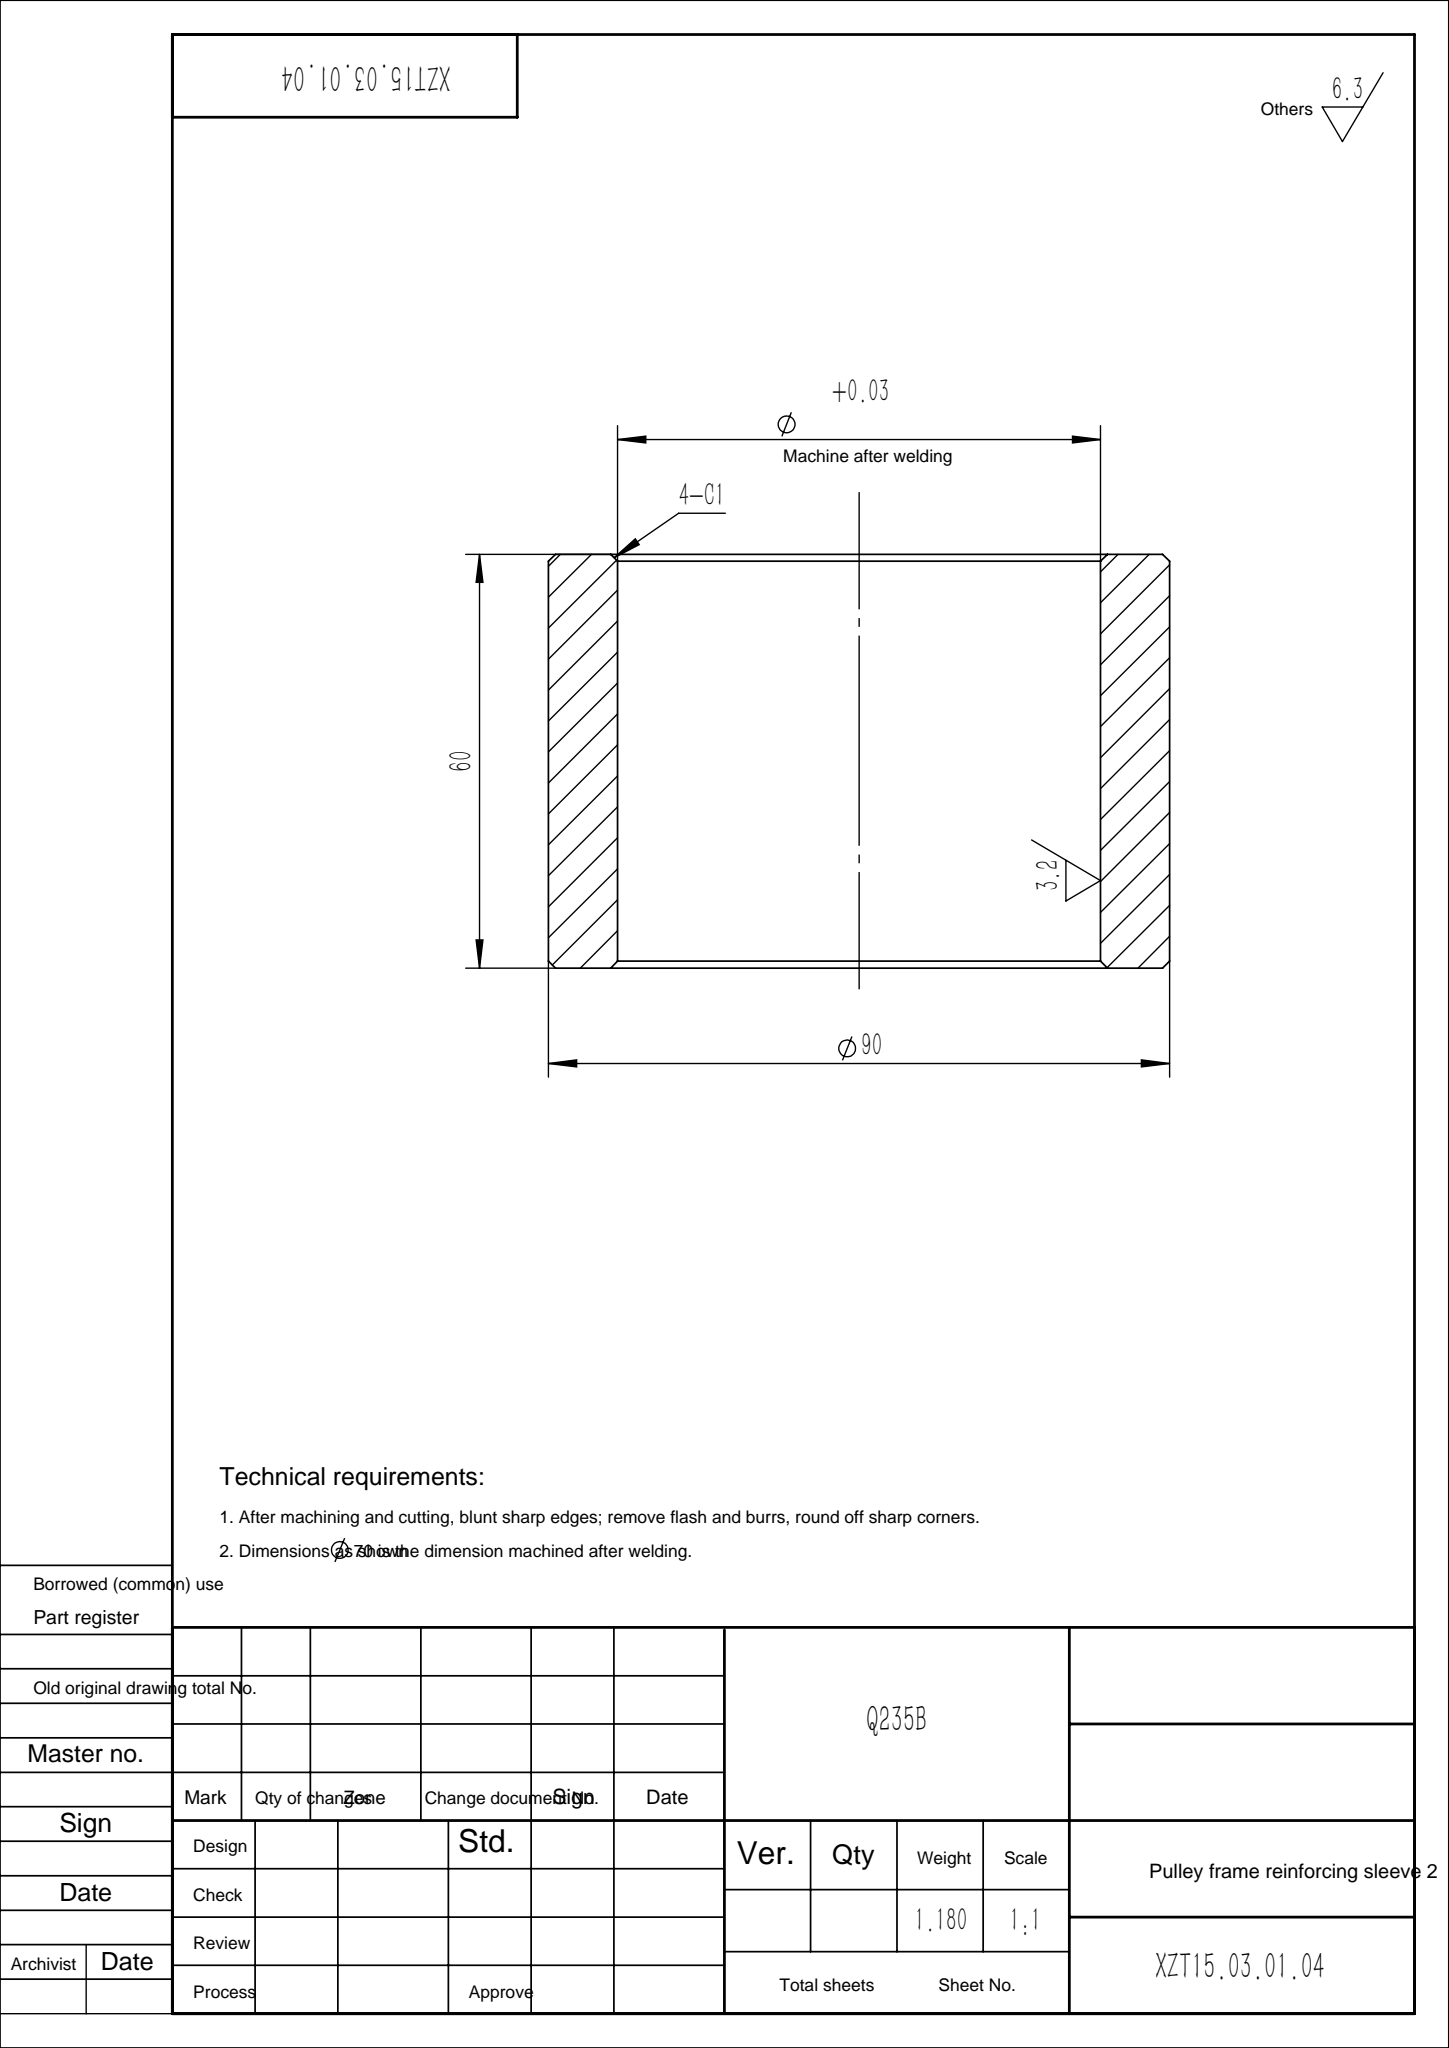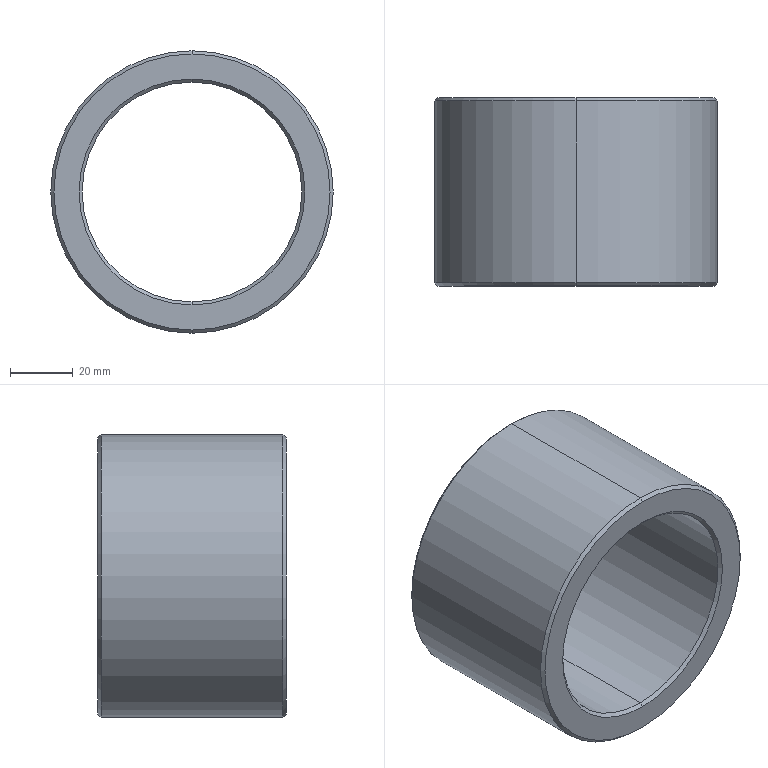Part | SolidWorks | features Chamfer 1, Extrusion 1 | 1 solid | 14 faces | box 90 x 60 x 90 mm | volume 150294 mm3 | cone 8 | cylinder 4 | plane 2 | commonest cylinder face diameters 70 x2 90 x2
STEP:
#1=CARTESIAN_POINT('',(0.,60.,44.));
#2=VERTEX_POINT('',#1);
#3=CARTESIAN_POINT('',(0.,60.,-44.));
#4=VERTEX_POINT('',#3);
#5=CARTESIAN_POINT('',(0.,60.,0.));
#6=DIRECTION('',(0.,1.,0.));
#7=DIRECTION('',(0.,0.,1.));
#8=AXIS2_PLACEMENT_3D('',#5,#6,#7);
#9=CIRCLE('',#8,44.);
#10=EDGE_CURVE('',#2,#4,#9,.T.);
#11=ORIENTED_EDGE('',*,*,#10,.F.);
#12=CARTESIAN_POINT('',(0.,59.,45.));
#13=VERTEX_POINT('',#12);
#14=CARTESIAN_POINT('',(0.,60.,44.));
#15=DIRECTION('',(0.,-0.7071,0.7071));
#16=VECTOR('',#15,1000.);
#17=LINE('',#14,#16);
#18=EDGE_CURVE('',#2,#13,#17,.T.);
#19=ORIENTED_EDGE('',*,*,#18,.T.);
#20=CARTESIAN_POINT('',(0.,59.,-45.));
#21=VERTEX_POINT('',#20);
#22=CARTESIAN_POINT('',(0.,59.,0.));
#23=DIRECTION('',(0.,-1.,0.));
#24=DIRECTION('',(0.,0.,1.));
#25=AXIS2_PLACEMENT_3D('',#22,#23,#24);
#26=CIRCLE('',#25,45.);
#27=EDGE_CURVE('',#21,#13,#26,.T.);
#28=ORIENTED_EDGE('',*,*,#27,.F.);
#29=CARTESIAN_POINT('',(0.,60.,-44.));
#30=DIRECTION('',(0.,-0.7071,-0.7071));
#31=VECTOR('',#30,1000.);
#32=LINE('',#29,#31);
#33=EDGE_CURVE('',#4,#21,#32,.T.);
#34=ORIENTED_EDGE('',*,*,#33,.F.);
#35=EDGE_LOOP('',(#11,#19,#28,#34));
#36=FACE_OUTER_BOUND('',#35,.T.);
#37=CARTESIAN_POINT('',(0.,60.,0.));
#38=DIRECTION('',(0.,-1.,0.));
#39=DIRECTION('',(0.,0.,-1.));
#40=AXIS2_PLACEMENT_3D('',#37,#38,#39);
#41=CONICAL_SURFACE('',#40,44.,0.7854);
#42=ADVANCED_FACE('',(#36),#41,.T.);
#43=CARTESIAN_POINT('',(0.,0.,-44.));
#44=VERTEX_POINT('',#43);
#45=CARTESIAN_POINT('',(0.,0.,44.));
#46=VERTEX_POINT('',#45);
#47=CARTESIAN_POINT('',(0.,0.,0.));
#48=DIRECTION('',(0.,-1.,0.));
#49=DIRECTION('',(0.,0.,1.));
#50=AXIS2_PLACEMENT_3D('',#47,#48,#49);
#51=CIRCLE('',#50,44.);
#52=EDGE_CURVE('',#44,#46,#51,.T.);
#53=ORIENTED_EDGE('',*,*,#52,.F.);
#54=CARTESIAN_POINT('',(0.,1.,-45.));
#55=VERTEX_POINT('',#54);
#56=CARTESIAN_POINT('',(0.,1.,-45.));
#57=DIRECTION('',(0.,0.7071,-0.7071));
#58=VECTOR('',#57,1000.);
#59=LINE('',#56,#58);
#60=EDGE_CURVE('',#44,#55,#59,.T.);
#61=ORIENTED_EDGE('',*,*,#60,.T.);
#62=CARTESIAN_POINT('',(0.,1.,45.));
#63=VERTEX_POINT('',#62);
#64=CARTESIAN_POINT('',(0.,1.,0.));
#65=DIRECTION('',(0.,1.,0.));
#66=DIRECTION('',(0.,0.,1.));
#67=AXIS2_PLACEMENT_3D('',#64,#65,#66);
#68=CIRCLE('',#67,45.);
#69=EDGE_CURVE('',#63,#55,#68,.T.);
#70=ORIENTED_EDGE('',*,*,#69,.F.);
#71=CARTESIAN_POINT('',(0.,1.,45.));
#72=DIRECTION('',(0.,0.7071,0.7071));
#73=VECTOR('',#72,1000.);
#74=LINE('',#71,#73);
#75=EDGE_CURVE('',#46,#63,#74,.T.);
#76=ORIENTED_EDGE('',*,*,#75,.F.);
#77=EDGE_LOOP('',(#53,#61,#70,#76));
#78=FACE_OUTER_BOUND('',#77,.T.);
#79=CARTESIAN_POINT('',(0.,1.,0.));
#80=DIRECTION('',(0.,1.,0.));
#81=DIRECTION('',(0.,0.,1.));
#82=AXIS2_PLACEMENT_3D('',#79,#80,#81);
#83=CONICAL_SURFACE('',#82,45.,0.7854);
#84=ADVANCED_FACE('',(#78),#83,.T.);
#85=CARTESIAN_POINT('',(0.,59.,-35.));
#86=VERTEX_POINT('',#85);
#87=CARTESIAN_POINT('',(0.,59.,35.));
#88=VERTEX_POINT('',#87);
#89=CARTESIAN_POINT('',(0.,59.,0.));
#90=DIRECTION('',(0.,1.,0.));
#91=DIRECTION('',(0.,0.,1.));
#92=AXIS2_PLACEMENT_3D('',#89,#90,#91);
#93=CIRCLE('',#92,35.);
#94=EDGE_CURVE('',#86,#88,#93,.T.);
#95=ORIENTED_EDGE('',*,*,#94,.F.);
#96=CARTESIAN_POINT('',(0.,60.,-36.));
#97=VERTEX_POINT('',#96);
#98=CARTESIAN_POINT('',(0.,59.,-35.));
#99=DIRECTION('',(0.,0.7071,-0.7071));
#100=VECTOR('',#99,1000.);
#101=LINE('',#98,#100);
#102=EDGE_CURVE('',#86,#97,#101,.T.);
#103=ORIENTED_EDGE('',*,*,#102,.T.);
#104=CARTESIAN_POINT('',(0.,60.,36.));
#105=VERTEX_POINT('',#104);
#106=CARTESIAN_POINT('',(0.,60.,0.));
#107=DIRECTION('',(0.,-1.,0.));
#108=DIRECTION('',(0.,0.,1.));
#109=AXIS2_PLACEMENT_3D('',#106,#107,#108);
#110=CIRCLE('',#109,36.);
#111=EDGE_CURVE('',#105,#97,#110,.T.);
#112=ORIENTED_EDGE('',*,*,#111,.F.);
#113=CARTESIAN_POINT('',(0.,59.,35.));
#114=DIRECTION('',(0.,0.7071,0.7071));
#115=VECTOR('',#114,1000.);
#116=LINE('',#113,#115);
#117=EDGE_CURVE('',#88,#105,#116,.T.);
#118=ORIENTED_EDGE('',*,*,#117,.F.);
#119=EDGE_LOOP('',(#95,#103,#112,#118));
#120=FACE_OUTER_BOUND('',#119,.T.);
#121=CARTESIAN_POINT('',(0.,59.,0.));
#122=DIRECTION('',(0.,1.,0.));
#123=DIRECTION('',(0.,0.,1.));
#124=AXIS2_PLACEMENT_3D('',#121,#122,#123);
#125=CONICAL_SURFACE('',#124,35.,0.7854);
#126=ADVANCED_FACE('',(#120),#125,.F.);
#127=CARTESIAN_POINT('',(0.,1.,35.));
#128=VERTEX_POINT('',#127);
#129=CARTESIAN_POINT('',(0.,1.,-35.));
#130=VERTEX_POINT('',#129);
#131=CARTESIAN_POINT('',(0.,1.,0.));
#132=DIRECTION('',(0.,-1.,0.));
#133=DIRECTION('',(0.,0.,1.));
#134=AXIS2_PLACEMENT_3D('',#131,#132,#133);
#135=CIRCLE('',#134,35.);
#136=EDGE_CURVE('',#128,#130,#135,.T.);
#137=ORIENTED_EDGE('',*,*,#136,.F.);
#138=CARTESIAN_POINT('',(0.,0.,36.));
#139=VERTEX_POINT('',#138);
#140=CARTESIAN_POINT('',(0.,0.,36.));
#141=DIRECTION('',(0.,-0.7071,0.7071));
#142=VECTOR('',#141,1000.);
#143=LINE('',#140,#142);
#144=EDGE_CURVE('',#128,#139,#143,.T.);
#145=ORIENTED_EDGE('',*,*,#144,.T.);
#146=CARTESIAN_POINT('',(0.,0.,-36.));
#147=VERTEX_POINT('',#146);
#148=CARTESIAN_POINT('',(0.,0.,0.));
#149=DIRECTION('',(0.,1.,0.));
#150=DIRECTION('',(0.,0.,1.));
#151=AXIS2_PLACEMENT_3D('',#148,#149,#150);
#152=CIRCLE('',#151,36.);
#153=EDGE_CURVE('',#147,#139,#152,.T.);
#154=ORIENTED_EDGE('',*,*,#153,.F.);
#155=CARTESIAN_POINT('',(0.,0.,-36.));
#156=DIRECTION('',(0.,-0.7071,-0.7071));
#157=VECTOR('',#156,1000.);
#158=LINE('',#155,#157);
#159=EDGE_CURVE('',#130,#147,#158,.T.);
#160=ORIENTED_EDGE('',*,*,#159,.F.);
#161=EDGE_LOOP('',(#137,#145,#154,#160));
#162=FACE_OUTER_BOUND('',#161,.T.);
#163=CARTESIAN_POINT('',(0.,0.,0.));
#164=DIRECTION('',(0.,-1.,0.));
#165=DIRECTION('',(0.,0.,-1.));
#166=AXIS2_PLACEMENT_3D('',#163,#164,#165);
#167=CONICAL_SURFACE('',#166,36.,0.7854);
#168=ADVANCED_FACE('',(#162),#167,.F.);
#169=ORIENTED_EDGE('',*,*,#94,.T.);
#170=CARTESIAN_POINT('',(0.,60.,35.));
#171=DIRECTION('',(0.,-1.,0.));
#172=VECTOR('',#171,1000.);
#173=LINE('',#170,#172);
#174=EDGE_CURVE('',#88,#128,#173,.T.);
#175=ORIENTED_EDGE('',*,*,#174,.T.);
#176=ORIENTED_EDGE('',*,*,#136,.T.);
#177=CARTESIAN_POINT('',(0.,60.,-35.));
#178=DIRECTION('',(0.,-1.,0.));
#179=VECTOR('',#178,1000.);
#180=LINE('',#177,#179);
#181=EDGE_CURVE('',#86,#130,#180,.T.);
#182=ORIENTED_EDGE('',*,*,#181,.F.);
#183=EDGE_LOOP('',(#169,#175,#176,#182));
#184=FACE_OUTER_BOUND('',#183,.T.);
#185=CARTESIAN_POINT('',(0.,60.,0.));
#186=DIRECTION('',(0.,-1.,0.));
#187=DIRECTION('',(0.,0.,-1.));
#188=AXIS2_PLACEMENT_3D('',#185,#186,#187);
#189=CYLINDRICAL_SURFACE('',#188,35.);
#190=ADVANCED_FACE('',(#184),#189,.F.);
#191=ORIENTED_EDGE('',*,*,#27,.T.);
#192=CARTESIAN_POINT('',(0.,60.,45.));
#193=DIRECTION('',(0.,-1.,0.));
#194=VECTOR('',#193,1000.);
#195=LINE('',#192,#194);
#196=EDGE_CURVE('',#13,#63,#195,.T.);
#197=ORIENTED_EDGE('',*,*,#196,.T.);
#198=ORIENTED_EDGE('',*,*,#69,.T.);
#199=CARTESIAN_POINT('',(0.,60.,-45.));
#200=DIRECTION('',(0.,-1.,0.));
#201=VECTOR('',#200,1000.);
#202=LINE('',#199,#201);
#203=EDGE_CURVE('',#21,#55,#202,.T.);
#204=ORIENTED_EDGE('',*,*,#203,.F.);
#205=EDGE_LOOP('',(#191,#197,#198,#204));
#206=FACE_OUTER_BOUND('',#205,.T.);
#207=CARTESIAN_POINT('',(0.,60.,0.));
#208=DIRECTION('',(0.,-1.,0.));
#209=DIRECTION('',(0.,0.,-1.));
#210=AXIS2_PLACEMENT_3D('',#207,#208,#209);
#211=CYLINDRICAL_SURFACE('',#210,45.);
#212=ADVANCED_FACE('',(#206),#211,.T.);
#213=ORIENTED_EDGE('',*,*,#111,.T.);
#214=CARTESIAN_POINT('',(0.,60.,0.));
#215=DIRECTION('',(0.,-1.,0.));
#216=DIRECTION('',(0.,0.,1.));
#217=AXIS2_PLACEMENT_3D('',#214,#215,#216);
#218=CIRCLE('',#217,36.);
#219=EDGE_CURVE('',#97,#105,#218,.T.);
#220=ORIENTED_EDGE('',*,*,#219,.T.);
#221=EDGE_LOOP('',(#213,#220));
#222=FACE_BOUND('',#221,.T.);
#223=CARTESIAN_POINT('',(0.,60.,0.));
#224=DIRECTION('',(0.,1.,0.));
#225=DIRECTION('',(0.,0.,1.));
#226=AXIS2_PLACEMENT_3D('',#223,#224,#225);
#227=CIRCLE('',#226,44.);
#228=EDGE_CURVE('',#4,#2,#227,.T.);
#229=ORIENTED_EDGE('',*,*,#228,.T.);
#230=ORIENTED_EDGE('',*,*,#10,.T.);
#231=EDGE_LOOP('',(#229,#230));
#232=FACE_OUTER_BOUND('',#231,.T.);
#233=CARTESIAN_POINT('',(0.,60.,0.));
#234=DIRECTION('',(0.,1.,0.));
#235=DIRECTION('',(0.,0.,1.));
#236=AXIS2_PLACEMENT_3D('',#233,#234,#235);
#237=PLANE('',#236);
#238=ADVANCED_FACE('',(#222,#232),#237,.T.);
#239=ORIENTED_EDGE('',*,*,#153,.T.);
#240=CARTESIAN_POINT('',(0.,0.,0.));
#241=DIRECTION('',(0.,1.,0.));
#242=DIRECTION('',(0.,0.,1.));
#243=AXIS2_PLACEMENT_3D('',#240,#241,#242);
#244=CIRCLE('',#243,36.);
#245=EDGE_CURVE('',#139,#147,#244,.T.);
#246=ORIENTED_EDGE('',*,*,#245,.T.);
#247=EDGE_LOOP('',(#239,#246));
#248=FACE_BOUND('',#247,.T.);
#249=CARTESIAN_POINT('',(0.,0.,0.));
#250=DIRECTION('',(0.,-1.,0.));
#251=DIRECTION('',(0.,0.,1.));
#252=AXIS2_PLACEMENT_3D('',#249,#250,#251);
#253=CIRCLE('',#252,44.);
#254=EDGE_CURVE('',#46,#44,#253,.T.);
#255=ORIENTED_EDGE('',*,*,#254,.T.);
#256=ORIENTED_EDGE('',*,*,#52,.T.);
#257=EDGE_LOOP('',(#255,#256));
#258=FACE_OUTER_BOUND('',#257,.T.);
#259=CARTESIAN_POINT('',(0.,0.,0.));
#260=DIRECTION('',(0.,1.,0.));
#261=DIRECTION('',(0.,0.,1.));
#262=AXIS2_PLACEMENT_3D('',#259,#260,#261);
#263=PLANE('',#262);
#264=ADVANCED_FACE('',(#248,#258),#263,.F.);
#265=ORIENTED_EDGE('',*,*,#196,.F.);
#266=CARTESIAN_POINT('',(0.,59.,0.));
#267=DIRECTION('',(0.,-1.,0.));
#268=DIRECTION('',(0.,0.,1.));
#269=AXIS2_PLACEMENT_3D('',#266,#267,#268);
#270=CIRCLE('',#269,45.);
#271=EDGE_CURVE('',#13,#21,#270,.T.);
#272=ORIENTED_EDGE('',*,*,#271,.T.);
#273=ORIENTED_EDGE('',*,*,#203,.T.);
#274=CARTESIAN_POINT('',(0.,1.,0.));
#275=DIRECTION('',(0.,1.,0.));
#276=DIRECTION('',(0.,0.,1.));
#277=AXIS2_PLACEMENT_3D('',#274,#275,#276);
#278=CIRCLE('',#277,45.);
#279=EDGE_CURVE('',#55,#63,#278,.T.);
#280=ORIENTED_EDGE('',*,*,#279,.T.);
#281=EDGE_LOOP('',(#265,#272,#273,#280));
#282=FACE_OUTER_BOUND('',#281,.T.);
#283=CARTESIAN_POINT('',(0.,60.,0.));
#284=DIRECTION('',(0.,-1.,0.));
#285=DIRECTION('',(0.,0.,-1.));
#286=AXIS2_PLACEMENT_3D('',#283,#284,#285);
#287=CYLINDRICAL_SURFACE('',#286,45.);
#288=ADVANCED_FACE('',(#282),#287,.T.);
#289=ORIENTED_EDGE('',*,*,#174,.F.);
#290=CARTESIAN_POINT('',(0.,59.,0.));
#291=DIRECTION('',(0.,1.,0.));
#292=DIRECTION('',(0.,0.,1.));
#293=AXIS2_PLACEMENT_3D('',#290,#291,#292);
#294=CIRCLE('',#293,35.);
#295=EDGE_CURVE('',#88,#86,#294,.T.);
#296=ORIENTED_EDGE('',*,*,#295,.T.);
#297=ORIENTED_EDGE('',*,*,#181,.T.);
#298=CARTESIAN_POINT('',(0.,1.,0.));
#299=DIRECTION('',(0.,-1.,0.));
#300=DIRECTION('',(0.,0.,1.));
#301=AXIS2_PLACEMENT_3D('',#298,#299,#300);
#302=CIRCLE('',#301,35.);
#303=EDGE_CURVE('',#130,#128,#302,.T.);
#304=ORIENTED_EDGE('',*,*,#303,.T.);
#305=EDGE_LOOP('',(#289,#296,#297,#304));
#306=FACE_OUTER_BOUND('',#305,.T.);
#307=CARTESIAN_POINT('',(0.,60.,0.));
#308=DIRECTION('',(0.,-1.,0.));
#309=DIRECTION('',(0.,0.,-1.));
#310=AXIS2_PLACEMENT_3D('',#307,#308,#309);
#311=CYLINDRICAL_SURFACE('',#310,35.);
#312=ADVANCED_FACE('',(#306),#311,.F.);
#313=ORIENTED_EDGE('',*,*,#144,.F.);
#314=ORIENTED_EDGE('',*,*,#303,.F.);
#315=ORIENTED_EDGE('',*,*,#159,.T.);
#316=ORIENTED_EDGE('',*,*,#245,.F.);
#317=EDGE_LOOP('',(#313,#314,#315,#316));
#318=FACE_OUTER_BOUND('',#317,.T.);
#319=CARTESIAN_POINT('',(0.,0.,0.));
#320=DIRECTION('',(0.,-1.,0.));
#321=DIRECTION('',(0.,0.,-1.));
#322=AXIS2_PLACEMENT_3D('',#319,#320,#321);
#323=CONICAL_SURFACE('',#322,36.,0.7854);
#324=ADVANCED_FACE('',(#318),#323,.F.);
#325=ORIENTED_EDGE('',*,*,#102,.F.);
#326=ORIENTED_EDGE('',*,*,#295,.F.);
#327=ORIENTED_EDGE('',*,*,#117,.T.);
#328=ORIENTED_EDGE('',*,*,#219,.F.);
#329=EDGE_LOOP('',(#325,#326,#327,#328));
#330=FACE_OUTER_BOUND('',#329,.T.);
#331=CARTESIAN_POINT('',(0.,59.,0.));
#332=DIRECTION('',(0.,1.,0.));
#333=DIRECTION('',(0.,0.,1.));
#334=AXIS2_PLACEMENT_3D('',#331,#332,#333);
#335=CONICAL_SURFACE('',#334,35.,0.7854);
#336=ADVANCED_FACE('',(#330),#335,.F.);
#337=ORIENTED_EDGE('',*,*,#60,.F.);
#338=ORIENTED_EDGE('',*,*,#254,.F.);
#339=ORIENTED_EDGE('',*,*,#75,.T.);
#340=ORIENTED_EDGE('',*,*,#279,.F.);
#341=EDGE_LOOP('',(#337,#338,#339,#340));
#342=FACE_OUTER_BOUND('',#341,.T.);
#343=CARTESIAN_POINT('',(0.,1.,0.));
#344=DIRECTION('',(0.,1.,0.));
#345=DIRECTION('',(0.,0.,1.));
#346=AXIS2_PLACEMENT_3D('',#343,#344,#345);
#347=CONICAL_SURFACE('',#346,45.,0.7854);
#348=ADVANCED_FACE('',(#342),#347,.T.);
#349=ORIENTED_EDGE('',*,*,#18,.F.);
#350=ORIENTED_EDGE('',*,*,#228,.F.);
#351=ORIENTED_EDGE('',*,*,#33,.T.);
#352=ORIENTED_EDGE('',*,*,#271,.F.);
#353=EDGE_LOOP('',(#349,#350,#351,#352));
#354=FACE_OUTER_BOUND('',#353,.T.);
#355=CARTESIAN_POINT('',(0.,60.,0.));
#356=DIRECTION('',(0.,-1.,0.));
#357=DIRECTION('',(0.,0.,-1.));
#358=AXIS2_PLACEMENT_3D('',#355,#356,#357);
#359=CONICAL_SURFACE('',#358,44.,0.7854);
#360=ADVANCED_FACE('',(#354),#359,.T.);
#361=CLOSED_SHELL('',(#42,#84,#126,#168,#190,#212,#238,#264,#288,#312,#324,#336,#348,#360));
#362=MANIFOLD_SOLID_BREP('',#361);
#363=CARTESIAN_POINT('',(0.,0.,0.));
#364=DIRECTION('',(0.,0.,1.));
#365=DIRECTION('',(1.,0.,0.));
#366=AXIS2_PLACEMENT_3D('',#363,#364,#365);
#367=(LENGTH_UNIT()NAMED_UNIT(*)SI_UNIT(.MILLI.,.METRE.));
#368=UNCERTAINTY_MEASURE_WITH_UNIT(LENGTH_MEASURE(0.00001),#367,'','');
#369=(NAMED_UNIT(*)PLANE_ANGLE_UNIT()SI_UNIT($,.RADIAN.));
#370=(NAMED_UNIT(*)SI_UNIT($,.STERADIAN.)SOLID_ANGLE_UNIT());
#371=(GEOMETRIC_REPRESENTATION_CONTEXT(3)GLOBAL_UNCERTAINTY_ASSIGNED_CONTEXT((#368))GLOBAL_UNIT_ASSIGNED_CONTEXT((#367,#369,#370))REPRESENTATION_CONTEXT('',''));
#372=ADVANCED_BREP_SHAPE_REPRESENTATION('',(#362,#366),#371);